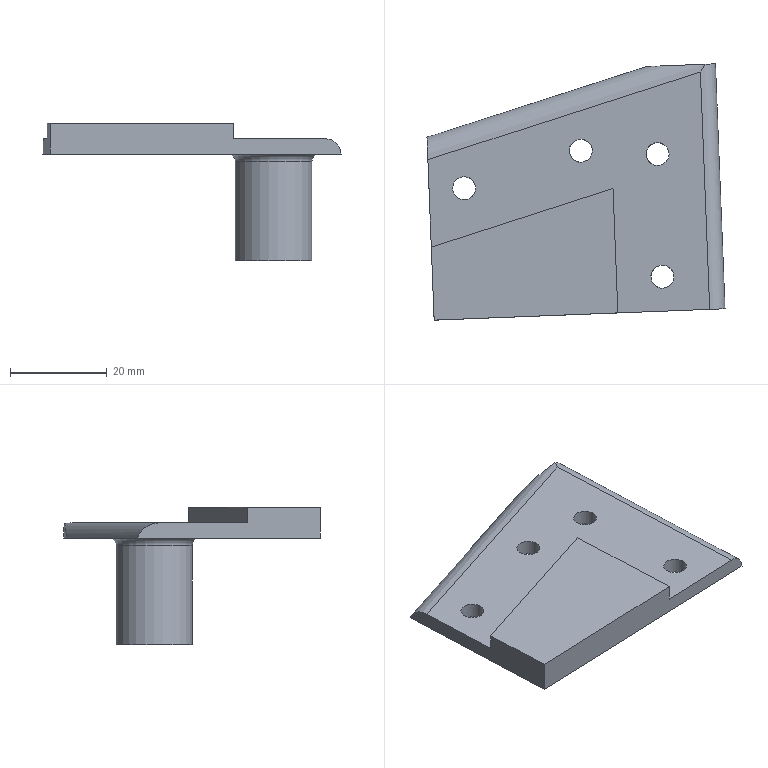Part | NX | features MG0301 nose pivot 24(left) 2 | 1 solid | 19 faces | box 61.764 x 53.123 x 28.4 mm | volume 14421 mm3 | plane 10 | cylinder 8 | torus 1 | commonest cylinder face diameters 4.763 x4 6.35 x2 9.525 x1 15.875 x1
STEP:
#1=CARTESIAN_POINT('',(-14.154,-41.859,-3.175));
#2=VERTEX_POINT('',#1);
#3=CARTESIAN_POINT('',(-14.154,-44.24,-3.175));
#4=DIRECTION('',(0.,0.,-1.));
#5=DIRECTION('',(0.,1.,0.));
#6=AXIS2_PLACEMENT_3D('',#3,#4,#5);
#7=CIRCLE('',#6,2.381);
#8=EDGE_CURVE('',#2,#2,#7,.T.);
#9=ORIENTED_EDGE('',*,*,#8,.T.);
#10=EDGE_LOOP('',(#9));
#11=FACE_BOUND('',#10,.T.);
#12=CARTESIAN_POINT('',(-55.242,-23.536,-3.175));
#13=VERTEX_POINT('',#12);
#14=CARTESIAN_POINT('',(-55.242,-25.917,-3.175));
#15=DIRECTION('',(0.,0.,-1.));
#16=DIRECTION('',(0.,1.,0.));
#17=AXIS2_PLACEMENT_3D('',#14,#15,#16);
#18=CIRCLE('',#17,2.381);
#19=EDGE_CURVE('',#13,#13,#18,.T.);
#20=ORIENTED_EDGE('',*,*,#19,.T.);
#21=EDGE_LOOP('',(#20));
#22=FACE_BOUND('',#21,.T.);
#23=CARTESIAN_POINT('',(-31.064,-15.754,-3.175));
#24=VERTEX_POINT('',#23);
#25=CARTESIAN_POINT('',(-31.064,-18.135,-3.175));
#26=DIRECTION('',(0.,0.,-1.));
#27=DIRECTION('',(0.,1.,0.));
#28=AXIS2_PLACEMENT_3D('',#25,#26,#27);
#29=CIRCLE('',#28,2.381);
#30=EDGE_CURVE('',#24,#24,#29,.T.);
#31=ORIENTED_EDGE('',*,*,#30,.T.);
#32=EDGE_LOOP('',(#31));
#33=FACE_BOUND('',#32,.T.);
#34=CARTESIAN_POINT('',(-15.149,-16.459,-3.175));
#35=VERTEX_POINT('',#34);
#36=CARTESIAN_POINT('',(-15.149,-18.84,-3.175));
#37=DIRECTION('',(0.,0.,-1.));
#38=DIRECTION('',(0.,1.,0.));
#39=AXIS2_PLACEMENT_3D('',#36,#37,#38);
#40=CIRCLE('',#39,2.381);
#41=EDGE_CURVE('',#35,#35,#40,.T.);
#42=ORIENTED_EDGE('',*,*,#41,.T.);
#43=EDGE_LOOP('',(#42));
#44=FACE_BOUND('',#43,.T.);
#45=CARTESIAN_POINT('',(-62.055,-38.116,-3.175));
#46=VERTEX_POINT('',#45);
#47=CARTESIAN_POINT('',(-24.401,-25.997,-3.175));
#48=VERTEX_POINT('',#47);
#49=CARTESIAN_POINT('',(-468.479,-168.921,-3.175));
#50=DIRECTION('',(0.9519,0.3064,0.));
#51=VECTOR('',#50,1000.);
#52=LINE('',#49,#51);
#53=EDGE_CURVE('',#46,#48,#52,.T.);
#54=ORIENTED_EDGE('',*,*,#53,.T.);
#55=CARTESIAN_POINT('',(-23.392,-51.755,-3.175));
#56=VERTEX_POINT('',#55);
#57=CARTESIAN_POINT('',(-5.139,-517.676,-3.175));
#58=DIRECTION('',(-0.03915,0.9992,0.));
#59=VECTOR('',#58,1000.);
#60=LINE('',#57,#59);
#61=EDGE_CURVE('',#56,#48,#60,.T.);
#62=ORIENTED_EDGE('',*,*,#61,.F.);
#63=CARTESIAN_POINT('',(-4.357,-51.01,-3.175));
#64=VERTEX_POINT('',#63);
#65=CARTESIAN_POINT('',(-61.463,-53.247,-3.175));
#66=DIRECTION('',(0.9992,0.03915,0.));
#67=VECTOR('',#66,1000.);
#68=LINE('',#65,#67);
#69=EDGE_CURVE('',#56,#64,#68,.T.);
#70=ORIENTED_EDGE('',*,*,#69,.T.);
#71=CARTESIAN_POINT('',(-6.284,-1.822,-3.175));
#72=VERTEX_POINT('',#71);
#73=CARTESIAN_POINT('',(13.897,-516.93,-3.175));
#74=DIRECTION('',(-0.03915,0.9992,0.));
#75=VECTOR('',#74,1000.);
#76=LINE('',#73,#75);
#77=EDGE_CURVE('',#64,#72,#76,.T.);
#78=ORIENTED_EDGE('',*,*,#77,.T.);
#79=CARTESIAN_POINT('',(-62.765,-20.,-3.175));
#80=VERTEX_POINT('',#79);
#81=CARTESIAN_POINT('',(-473.829,-152.298,-3.175));
#82=DIRECTION('',(0.9519,0.3064,0.));
#83=VECTOR('',#82,1000.);
#84=LINE('',#81,#83);
#85=EDGE_CURVE('',#80,#72,#84,.T.);
#86=ORIENTED_EDGE('',*,*,#85,.F.);
#87=CARTESIAN_POINT('',(-62.959,-15.059,-3.175));
#88=DIRECTION('',(0.03915,-0.9992,0.));
#89=VECTOR('',#88,1000.);
#90=LINE('',#87,#89);
#91=EDGE_CURVE('',#80,#46,#90,.T.);
#92=ORIENTED_EDGE('',*,*,#91,.T.);
#93=EDGE_LOOP('',(#54,#62,#70,#78,#86,#92));
#94=FACE_BOUND('',#93,.T.);
#95=CARTESIAN_POINT('',(-468.479,-168.921,-3.175));
#96=DIRECTION('',(0.,0.,-1.));
#97=DIRECTION('',(0.,1.,0.));
#98=AXIS2_PLACEMENT_3D('',#95,#96,#97);
#99=PLANE('',#98);
#100=ADVANCED_FACE('',(#11,#22,#33,#44,#94),#99,.F.);
#101=CARTESIAN_POINT('',(-3.173,-0.1243,-6.35));
#102=VERTEX_POINT('',#101);
#103=CARTESIAN_POINT('',(-5.334,-0.209,-3.34));
#104=VERTEX_POINT('',#103);
#105=CARTESIAN_POINT('',(-6.345,-0.2486,-6.35));
#106=DIRECTION('',(-0.03915,0.9992,0.));
#107=DIRECTION('',(-0.9992,-0.03915,0.));
#108=AXIS2_PLACEMENT_3D('',#105,#106,#107);
#109=CIRCLE('',#108,3.175);
#110=EDGE_CURVE('',#102,#104,#109,.F.);
#111=ORIENTED_EDGE('',*,*,#110,.F.);
#112=CARTESIAN_POINT('',(-17.397,-0.6816,-6.35));
#113=VERTEX_POINT('',#112);
#114=CARTESIAN_POINT('',(0.,0.,-6.35));
#115=DIRECTION('',(-0.9992,-0.03915,0.));
#116=VECTOR('',#115,1000.);
#117=LINE('',#114,#116);
#118=EDGE_CURVE('',#102,#113,#117,.T.);
#119=ORIENTED_EDGE('',*,*,#118,.T.);
#120=CARTESIAN_POINT('',(-0.7099,-0.02781,-7.938));
#121=DIRECTION('',(-0.03915,0.9992,0.));
#122=DIRECTION('',(0.9992,0.03915,0.));
#123=AXIS2_PLACEMENT_3D('',#120,#121,#122);
#124=ELLIPSE('',#123,17.713,4.763);
#125=EDGE_CURVE('',#104,#113,#124,.F.);
#126=ORIENTED_EDGE('',*,*,#125,.F.);
#127=EDGE_LOOP('',(#111,#119,#126));
#128=FACE_BOUND('',#127,.T.);
#129=CARTESIAN_POINT('',(0.,0.,-6.35));
#130=DIRECTION('',(-0.03915,0.9992,0.));
#131=DIRECTION('',(-0.9992,-0.03915,0.));
#132=AXIS2_PLACEMENT_3D('',#129,#130,#131);
#133=PLANE('',#132);
#134=ADVANCED_FACE('',(#128),#133,.T.);
#135=CARTESIAN_POINT('',(-23.392,-51.755,0.));
#136=VERTEX_POINT('',#135);
#137=CARTESIAN_POINT('',(-23.392,-51.755,-6.35));
#138=DIRECTION('',(0.,0.,-1.));
#139=VECTOR('',#138,1000.);
#140=LINE('',#137,#139);
#141=EDGE_CURVE('',#136,#56,#140,.T.);
#142=ORIENTED_EDGE('',*,*,#141,.F.);
#143=CARTESIAN_POINT('',(-61.463,-53.247,0.));
#144=VERTEX_POINT('',#143);
#145=CARTESIAN_POINT('',(-61.463,-53.247,0.));
#146=DIRECTION('',(0.9992,0.03915,0.));
#147=VECTOR('',#146,1000.);
#148=LINE('',#145,#147);
#149=EDGE_CURVE('',#144,#136,#148,.T.);
#150=ORIENTED_EDGE('',*,*,#149,.F.);
#151=CARTESIAN_POINT('',(-61.463,-53.247,-6.35));
#152=VERTEX_POINT('',#151);
#153=CARTESIAN_POINT('',(-61.463,-53.247,-6.35));
#154=DIRECTION('',(0.,0.,1.));
#155=VECTOR('',#154,1000.);
#156=LINE('',#153,#155);
#157=EDGE_CURVE('',#152,#144,#156,.T.);
#158=ORIENTED_EDGE('',*,*,#157,.F.);
#159=CARTESIAN_POINT('',(-1.184,-50.885,-6.35));
#160=VERTEX_POINT('',#159);
#161=CARTESIAN_POINT('',(-61.463,-53.247,-6.35));
#162=DIRECTION('',(0.9992,0.03915,0.));
#163=VECTOR('',#162,1000.);
#164=LINE('',#161,#163);
#165=EDGE_CURVE('',#152,#160,#164,.T.);
#166=ORIENTED_EDGE('',*,*,#165,.T.);
#167=CARTESIAN_POINT('',(-4.357,-51.01,-6.35));
#168=DIRECTION('',(0.03915,-0.9992,0.));
#169=DIRECTION('',(0.9992,0.03915,0.));
#170=AXIS2_PLACEMENT_3D('',#167,#168,#169);
#171=CIRCLE('',#170,3.175);
#172=EDGE_CURVE('',#64,#160,#171,.F.);
#173=ORIENTED_EDGE('',*,*,#172,.F.);
#174=ORIENTED_EDGE('',*,*,#69,.F.);
#175=EDGE_LOOP('',(#142,#150,#158,#166,#173,#174));
#176=FACE_BOUND('',#175,.T.);
#177=CARTESIAN_POINT('',(-61.463,-53.247,-6.35));
#178=DIRECTION('',(0.03915,-0.9992,0.));
#179=DIRECTION('',(0.9992,0.03915,0.));
#180=AXIS2_PLACEMENT_3D('',#177,#178,#179);
#181=PLANE('',#180);
#182=ADVANCED_FACE('',(#176),#181,.T.);
#183=CARTESIAN_POINT('',(-62.948,-15.342,-6.35));
#184=VERTEX_POINT('',#183);
#185=CARTESIAN_POINT('',(-62.765,-20.,-7.938));
#186=DIRECTION('',(-0.9992,-0.03915,0.));
#187=DIRECTION('',(-0.03915,0.9992,0.));
#188=AXIS2_PLACEMENT_3D('',#185,#186,#187);
#189=ELLIPSE('',#188,4.945,4.763);
#190=EDGE_CURVE('',#184,#80,#189,.F.);
#191=ORIENTED_EDGE('',*,*,#190,.F.);
#192=CARTESIAN_POINT('',(-62.959,-15.059,-6.35));
#193=DIRECTION('',(0.03915,-0.9992,0.));
#194=VECTOR('',#193,1000.);
#195=LINE('',#192,#194);
#196=EDGE_CURVE('',#184,#152,#195,.T.);
#197=ORIENTED_EDGE('',*,*,#196,.T.);
#198=ORIENTED_EDGE('',*,*,#157,.T.);
#199=CARTESIAN_POINT('',(-62.055,-38.116,0.));
#200=VERTEX_POINT('',#199);
#201=CARTESIAN_POINT('',(-62.959,-15.059,0.));
#202=DIRECTION('',(0.03915,-0.9992,0.));
#203=VECTOR('',#202,1000.);
#204=LINE('',#201,#203);
#205=EDGE_CURVE('',#200,#144,#204,.T.);
#206=ORIENTED_EDGE('',*,*,#205,.F.);
#207=CARTESIAN_POINT('',(-62.055,-38.116,-6.35));
#208=DIRECTION('',(0.,0.,1.));
#209=VECTOR('',#208,1000.);
#210=LINE('',#207,#209);
#211=EDGE_CURVE('',#46,#200,#210,.T.);
#212=ORIENTED_EDGE('',*,*,#211,.F.);
#213=ORIENTED_EDGE('',*,*,#91,.F.);
#214=EDGE_LOOP('',(#191,#197,#198,#206,#212,#213));
#215=FACE_BOUND('',#214,.T.);
#216=CARTESIAN_POINT('',(-62.959,-15.059,-6.35));
#217=DIRECTION('',(-0.9992,-0.03915,0.));
#218=DIRECTION('',(0.03915,-0.9992,0.));
#219=AXIS2_PLACEMENT_3D('',#216,#217,#218);
#220=PLANE('',#219);
#221=ADVANCED_FACE('',(#215),#220,.T.);
#222=CARTESIAN_POINT('',(-11.773,-44.24,-6.35));
#223=VERTEX_POINT('',#222);
#224=CARTESIAN_POINT('',(-14.154,-44.24,-6.35));
#225=DIRECTION('',(0.,0.,1.));
#226=DIRECTION('',(1.,0.,0.));
#227=AXIS2_PLACEMENT_3D('',#224,#225,#226);
#228=CIRCLE('',#227,2.381);
#229=EDGE_CURVE('',#223,#223,#228,.T.);
#230=ORIENTED_EDGE('',*,*,#229,.T.);
#231=EDGE_LOOP('',(#230));
#232=FACE_BOUND('',#231,.T.);
#233=CARTESIAN_POINT('',(-52.861,-25.917,-6.35));
#234=VERTEX_POINT('',#233);
#235=CARTESIAN_POINT('',(-55.242,-25.917,-6.35));
#236=DIRECTION('',(0.,0.,1.));
#237=DIRECTION('',(1.,0.,0.));
#238=AXIS2_PLACEMENT_3D('',#235,#236,#237);
#239=CIRCLE('',#238,2.381);
#240=EDGE_CURVE('',#234,#234,#239,.T.);
#241=ORIENTED_EDGE('',*,*,#240,.T.);
#242=EDGE_LOOP('',(#241));
#243=FACE_BOUND('',#242,.T.);
#244=CARTESIAN_POINT('',(-28.683,-18.135,-6.35));
#245=VERTEX_POINT('',#244);
#246=CARTESIAN_POINT('',(-31.064,-18.135,-6.35));
#247=DIRECTION('',(0.,0.,1.));
#248=DIRECTION('',(1.,0.,0.));
#249=AXIS2_PLACEMENT_3D('',#246,#247,#248);
#250=CIRCLE('',#249,2.381);
#251=EDGE_CURVE('',#245,#245,#250,.T.);
#252=ORIENTED_EDGE('',*,*,#251,.T.);
#253=EDGE_LOOP('',(#252));
#254=FACE_BOUND('',#253,.T.);
#255=CARTESIAN_POINT('',(-5.637,-18.84,-6.35));
#256=VERTEX_POINT('',#255);
#257=CARTESIAN_POINT('',(-15.149,-18.84,-6.35));
#258=DIRECTION('',(0.,0.,1.));
#259=DIRECTION('',(1.,0.,0.));
#260=AXIS2_PLACEMENT_3D('',#257,#258,#259);
#261=CIRCLE('',#260,9.512);
#262=EDGE_CURVE('',#256,#256,#261,.T.);
#263=ORIENTED_EDGE('',*,*,#262,.T.);
#264=EDGE_LOOP('',(#263));
#265=FACE_BOUND('',#264,.T.);
#266=ORIENTED_EDGE('',*,*,#118,.F.);
#267=CARTESIAN_POINT('',(17.069,-516.806,-6.35));
#268=DIRECTION('',(-0.03915,0.9992,0.));
#269=VECTOR('',#268,1000.);
#270=LINE('',#267,#269);
#271=EDGE_CURVE('',#160,#102,#270,.T.);
#272=ORIENTED_EDGE('',*,*,#271,.F.);
#273=ORIENTED_EDGE('',*,*,#165,.F.);
#274=ORIENTED_EDGE('',*,*,#196,.F.);
#275=CARTESIAN_POINT('',(-475.205,-148.024,-6.35));
#276=DIRECTION('',(0.9519,0.3064,0.));
#277=VECTOR('',#276,1000.);
#278=LINE('',#275,#277);
#279=EDGE_CURVE('',#184,#113,#278,.T.);
#280=ORIENTED_EDGE('',*,*,#279,.T.);
#281=EDGE_LOOP('',(#266,#272,#273,#274,#280));
#282=FACE_BOUND('',#281,.T.);
#283=CARTESIAN_POINT('',(-63.451,-2.486,-6.35));
#284=DIRECTION('',(0.,0.,1.));
#285=DIRECTION('',(1.,0.,0.));
#286=AXIS2_PLACEMENT_3D('',#283,#284,#285);
#287=PLANE('',#286);
#288=ADVANCED_FACE('',(#232,#243,#254,#265,#282),#287,.F.);
#289=CARTESIAN_POINT('',(-24.401,-25.997,0.));
#290=VERTEX_POINT('',#289);
#291=CARTESIAN_POINT('',(-5.139,-517.676,0.));
#292=DIRECTION('',(-0.03915,0.9992,0.));
#293=VECTOR('',#292,1000.);
#294=LINE('',#291,#293);
#295=EDGE_CURVE('',#136,#290,#294,.T.);
#296=ORIENTED_EDGE('',*,*,#295,.T.);
#297=CARTESIAN_POINT('',(-52.929,-35.179,0.));
#298=DIRECTION('',(0.9519,0.3064,0.));
#299=VECTOR('',#298,1000.);
#300=LINE('',#297,#299);
#301=EDGE_CURVE('',#200,#290,#300,.T.);
#302=ORIENTED_EDGE('',*,*,#301,.F.);
#303=ORIENTED_EDGE('',*,*,#205,.T.);
#304=ORIENTED_EDGE('',*,*,#149,.T.);
#305=EDGE_LOOP('',(#296,#302,#303,#304));
#306=FACE_BOUND('',#305,.T.);
#307=CARTESIAN_POINT('',(-63.451,-2.486,0.));
#308=DIRECTION('',(0.,0.,1.));
#309=DIRECTION('',(1.,0.,0.));
#310=AXIS2_PLACEMENT_3D('',#307,#308,#309);
#311=PLANE('',#310);
#312=ADVANCED_FACE('',(#306),#311,.T.);
#313=CARTESIAN_POINT('',(-7.212,-18.84,-7.925));
#314=VERTEX_POINT('',#313);
#315=CARTESIAN_POINT('',(-15.149,-18.84,-7.925));
#316=DIRECTION('',(0.,0.,1.));
#317=DIRECTION('',(1.,0.,0.));
#318=AXIS2_PLACEMENT_3D('',#315,#316,#317);
#319=CIRCLE('',#318,7.938);
#320=EDGE_CURVE('',#314,#314,#319,.F.);
#321=ORIENTED_EDGE('',*,*,#320,.T.);
#322=EDGE_LOOP('',(#321));
#323=FACE_BOUND('',#322,.T.);
#324=CARTESIAN_POINT('',(-7.212,-18.84,-28.4));
#325=VERTEX_POINT('',#324);
#326=CARTESIAN_POINT('',(-15.149,-18.84,-28.4));
#327=DIRECTION('',(0.,0.,1.));
#328=DIRECTION('',(1.,0.,0.));
#329=AXIS2_PLACEMENT_3D('',#326,#327,#328);
#330=CIRCLE('',#329,7.938);
#331=EDGE_CURVE('',#325,#325,#330,.T.);
#332=ORIENTED_EDGE('',*,*,#331,.T.);
#333=EDGE_LOOP('',(#332));
#334=FACE_BOUND('',#333,.T.);
#335=CARTESIAN_POINT('',(-15.149,-18.84,-25.4));
#336=DIRECTION('',(0.,0.,1.));
#337=DIRECTION('',(1.,0.,0.));
#338=AXIS2_PLACEMENT_3D('',#335,#336,#337);
#339=CYLINDRICAL_SURFACE('',#338,7.938);
#340=ADVANCED_FACE('',(#323,#334),#339,.T.);
#341=CARTESIAN_POINT('',(-11.974,-18.84,-28.4));
#342=VERTEX_POINT('',#341);
#343=CARTESIAN_POINT('',(-15.149,-18.84,-28.4));
#344=DIRECTION('',(0.,0.,1.));
#345=DIRECTION('',(1.,0.,0.));
#346=AXIS2_PLACEMENT_3D('',#343,#344,#345);
#347=CIRCLE('',#346,3.175);
#348=EDGE_CURVE('',#342,#342,#347,.T.);
#349=ORIENTED_EDGE('',*,*,#348,.F.);
#350=EDGE_LOOP('',(#349));
#351=FACE_BOUND('',#350,.T.);
#352=CARTESIAN_POINT('',(-11.974,-18.84,-6.35));
#353=VERTEX_POINT('',#352);
#354=CARTESIAN_POINT('',(-15.149,-18.84,-6.35));
#355=DIRECTION('',(0.,0.,1.));
#356=DIRECTION('',(1.,0.,0.));
#357=AXIS2_PLACEMENT_3D('',#354,#355,#356);
#358=CIRCLE('',#357,3.175);
#359=EDGE_CURVE('',#353,#353,#358,.T.);
#360=ORIENTED_EDGE('',*,*,#359,.T.);
#361=EDGE_LOOP('',(#360));
#362=FACE_BOUND('',#361,.T.);
#363=CARTESIAN_POINT('',(-15.149,-18.84,-25.4));
#364=DIRECTION('',(0.,0.,1.));
#365=DIRECTION('',(1.,0.,0.));
#366=AXIS2_PLACEMENT_3D('',#363,#364,#365);
#367=CYLINDRICAL_SURFACE('',#366,3.175);
#368=ADVANCED_FACE('',(#351,#362),#367,.F.);
#369=ORIENTED_EDGE('',*,*,#348,.T.);
#370=EDGE_LOOP('',(#369));
#371=FACE_BOUND('',#370,.T.);
#372=ORIENTED_EDGE('',*,*,#331,.F.);
#373=EDGE_LOOP('',(#372));
#374=FACE_BOUND('',#373,.T.);
#375=CARTESIAN_POINT('',(-15.149,-18.84,-28.4));
#376=DIRECTION('',(0.,0.,1.));
#377=DIRECTION('',(1.,0.,0.));
#378=AXIS2_PLACEMENT_3D('',#375,#376,#377);
#379=PLANE('',#378);
#380=ADVANCED_FACE('',(#371,#374),#379,.F.);
#381=CARTESIAN_POINT('',(-12.768,-18.84,-6.35));
#382=VERTEX_POINT('',#381);
#383=CARTESIAN_POINT('',(-15.149,-18.84,-6.35));
#384=DIRECTION('',(0.,0.,1.));
#385=DIRECTION('',(1.,0.,0.));
#386=AXIS2_PLACEMENT_3D('',#383,#384,#385);
#387=CIRCLE('',#386,2.381);
#388=EDGE_CURVE('',#382,#382,#387,.T.);
#389=ORIENTED_EDGE('',*,*,#388,.T.);
#390=EDGE_LOOP('',(#389));
#391=FACE_BOUND('',#390,.T.);
#392=ORIENTED_EDGE('',*,*,#359,.F.);
#393=EDGE_LOOP('',(#392));
#394=FACE_BOUND('',#393,.T.);
#395=CARTESIAN_POINT('',(-63.451,-2.486,-6.35));
#396=DIRECTION('',(0.,0.,1.));
#397=DIRECTION('',(1.,0.,0.));
#398=AXIS2_PLACEMENT_3D('',#395,#396,#397);
#399=PLANE('',#398);
#400=ADVANCED_FACE('',(#391,#394),#399,.F.);
#401=ORIENTED_EDGE('',*,*,#320,.F.);
#402=EDGE_LOOP('',(#401));
#403=FACE_BOUND('',#402,.T.);
#404=ORIENTED_EDGE('',*,*,#262,.F.);
#405=EDGE_LOOP('',(#404));
#406=FACE_BOUND('',#405,.T.);
#407=CARTESIAN_POINT('',(-15.149,-18.84,-7.925));
#408=DIRECTION('',(0.,0.,1.));
#409=DIRECTION('',(1.,0.,0.));
#410=AXIS2_PLACEMENT_3D('',#407,#408,#409);
#411=TOROIDAL_SURFACE('',#410,9.512,1.575);
#412=ADVANCED_FACE('',(#403,#406),#411,.F.);
#413=ORIENTED_EDGE('',*,*,#85,.T.);
#414=CARTESIAN_POINT('',(-5.334,-0.209,-3.34));
#415=CARTESIAN_POINT('',(-5.645,-0.741,-3.229));
#416=CARTESIAN_POINT('',(-5.964,-1.281,-3.175));
#417=CARTESIAN_POINT('',(-6.284,-1.822,-3.175));
#418=B_SPLINE_CURVE_WITH_KNOTS('',3,(#414,#415,#416,#417),.UNSPECIFIED.,.F.,.F.,(4,4),(0.005677,0.007559),.UNSPECIFIED.);
#419=EDGE_CURVE('',#72,#104,#418,.F.);
#420=ORIENTED_EDGE('',*,*,#419,.T.);
#421=ORIENTED_EDGE('',*,*,#125,.T.);
#422=ORIENTED_EDGE('',*,*,#279,.F.);
#423=ORIENTED_EDGE('',*,*,#190,.T.);
#424=EDGE_LOOP('',(#413,#420,#421,#422,#423));
#425=FACE_BOUND('',#424,.T.);
#426=CARTESIAN_POINT('',(-473.829,-152.298,-7.938));
#427=DIRECTION('',(0.9519,0.3064,0.));
#428=DIRECTION('',(-0.3064,0.9519,0.));
#429=AXIS2_PLACEMENT_3D('',#426,#427,#428);
#430=CYLINDRICAL_SURFACE('',#429,4.763);
#431=ADVANCED_FACE('',(#425),#430,.T.);
#432=ORIENTED_EDGE('',*,*,#301,.T.);
#433=CARTESIAN_POINT('',(-24.401,-25.997,0.));
#434=DIRECTION('',(0.,0.,-1.));
#435=VECTOR('',#434,1000.);
#436=LINE('',#433,#435);
#437=EDGE_CURVE('',#290,#48,#436,.T.);
#438=ORIENTED_EDGE('',*,*,#437,.T.);
#439=ORIENTED_EDGE('',*,*,#53,.F.);
#440=ORIENTED_EDGE('',*,*,#211,.T.);
#441=EDGE_LOOP('',(#432,#438,#439,#440));
#442=FACE_BOUND('',#441,.T.);
#443=CARTESIAN_POINT('',(-468.479,-168.921,0.));
#444=DIRECTION('',(0.3064,-0.9519,0.));
#445=DIRECTION('',(0.9519,0.3064,0.));
#446=AXIS2_PLACEMENT_3D('',#443,#444,#445);
#447=PLANE('',#446);
#448=ADVANCED_FACE('',(#442),#447,.F.);
#449=ORIENTED_EDGE('',*,*,#141,.T.);
#450=ORIENTED_EDGE('',*,*,#61,.T.);
#451=ORIENTED_EDGE('',*,*,#437,.F.);
#452=ORIENTED_EDGE('',*,*,#295,.F.);
#453=EDGE_LOOP('',(#449,#450,#451,#452));
#454=FACE_BOUND('',#453,.T.);
#455=CARTESIAN_POINT('',(-5.139,-517.676,0.));
#456=DIRECTION('',(-0.9992,-0.03915,0.));
#457=DIRECTION('',(0.03915,-0.9992,0.));
#458=AXIS2_PLACEMENT_3D('',#455,#456,#457);
#459=PLANE('',#458);
#460=ADVANCED_FACE('',(#454),#459,.F.);
#461=ORIENTED_EDGE('',*,*,#172,.T.);
#462=ORIENTED_EDGE('',*,*,#271,.T.);
#463=ORIENTED_EDGE('',*,*,#110,.T.);
#464=ORIENTED_EDGE('',*,*,#419,.F.);
#465=ORIENTED_EDGE('',*,*,#77,.F.);
#466=EDGE_LOOP('',(#461,#462,#463,#464,#465));
#467=FACE_BOUND('',#466,.T.);
#468=CARTESIAN_POINT('',(13.897,-516.93,-6.35));
#469=DIRECTION('',(-0.03915,0.9992,0.));
#470=DIRECTION('',(-0.9992,-0.03915,0.));
#471=AXIS2_PLACEMENT_3D('',#468,#469,#470);
#472=CYLINDRICAL_SURFACE('',#471,3.175);
#473=ADVANCED_FACE('',(#467),#472,.T.);
#474=ORIENTED_EDGE('',*,*,#388,.F.);
#475=EDGE_LOOP('',(#474));
#476=FACE_BOUND('',#475,.T.);
#477=ORIENTED_EDGE('',*,*,#41,.F.);
#478=EDGE_LOOP('',(#477));
#479=FACE_BOUND('',#478,.T.);
#480=CARTESIAN_POINT('',(-15.149,-18.84,-63.5));
#481=DIRECTION('',(0.,0.,1.));
#482=DIRECTION('',(1.,0.,0.));
#483=AXIS2_PLACEMENT_3D('',#480,#481,#482);
#484=CYLINDRICAL_SURFACE('',#483,2.381);
#485=ADVANCED_FACE('',(#476,#479),#484,.F.);
#486=ORIENTED_EDGE('',*,*,#251,.F.);
#487=EDGE_LOOP('',(#486));
#488=FACE_BOUND('',#487,.T.);
#489=ORIENTED_EDGE('',*,*,#30,.F.);
#490=EDGE_LOOP('',(#489));
#491=FACE_BOUND('',#490,.T.);
#492=CARTESIAN_POINT('',(-31.064,-18.135,-63.5));
#493=DIRECTION('',(0.,0.,1.));
#494=DIRECTION('',(1.,0.,0.));
#495=AXIS2_PLACEMENT_3D('',#492,#493,#494);
#496=CYLINDRICAL_SURFACE('',#495,2.381);
#497=ADVANCED_FACE('',(#488,#491),#496,.F.);
#498=ORIENTED_EDGE('',*,*,#240,.F.);
#499=EDGE_LOOP('',(#498));
#500=FACE_BOUND('',#499,.T.);
#501=ORIENTED_EDGE('',*,*,#19,.F.);
#502=EDGE_LOOP('',(#501));
#503=FACE_BOUND('',#502,.T.);
#504=CARTESIAN_POINT('',(-55.242,-25.917,-63.5));
#505=DIRECTION('',(0.,0.,1.));
#506=DIRECTION('',(1.,0.,0.));
#507=AXIS2_PLACEMENT_3D('',#504,#505,#506);
#508=CYLINDRICAL_SURFACE('',#507,2.381);
#509=ADVANCED_FACE('',(#500,#503),#508,.F.);
#510=ORIENTED_EDGE('',*,*,#229,.F.);
#511=EDGE_LOOP('',(#510));
#512=FACE_BOUND('',#511,.T.);
#513=ORIENTED_EDGE('',*,*,#8,.F.);
#514=EDGE_LOOP('',(#513));
#515=FACE_BOUND('',#514,.T.);
#516=CARTESIAN_POINT('',(-14.154,-44.24,-63.5));
#517=DIRECTION('',(0.,0.,1.));
#518=DIRECTION('',(1.,0.,0.));
#519=AXIS2_PLACEMENT_3D('',#516,#517,#518);
#520=CYLINDRICAL_SURFACE('',#519,2.381);
#521=ADVANCED_FACE('',(#512,#515),#520,.F.);
#522=CLOSED_SHELL('',(#100,#134,#182,#221,#288,#312,#340,#368,#380,#400,#412,#431,#448,#460,#473,#485,#497,#509,#521));
#523=MANIFOLD_SOLID_BREP('',#522);
#524=(LENGTH_UNIT()NAMED_UNIT(*)SI_UNIT(.MILLI.,.METRE.));
#525=UNCERTAINTY_MEASURE_WITH_UNIT(LENGTH_MEASURE(0.0508),#524,'','');
#526=(NAMED_UNIT(*)PLANE_ANGLE_UNIT()SI_UNIT($,.RADIAN.));
#527=(NAMED_UNIT(*)SI_UNIT($,.STERADIAN.)SOLID_ANGLE_UNIT());
#528=(GEOMETRIC_REPRESENTATION_CONTEXT(3)GLOBAL_UNCERTAINTY_ASSIGNED_CONTEXT((#525))GLOBAL_UNIT_ASSIGNED_CONTEXT((#524,#526,#527))REPRESENTATION_CONTEXT('',''));
#529=ADVANCED_BREP_SHAPE_REPRESENTATION('',(#523),#528);